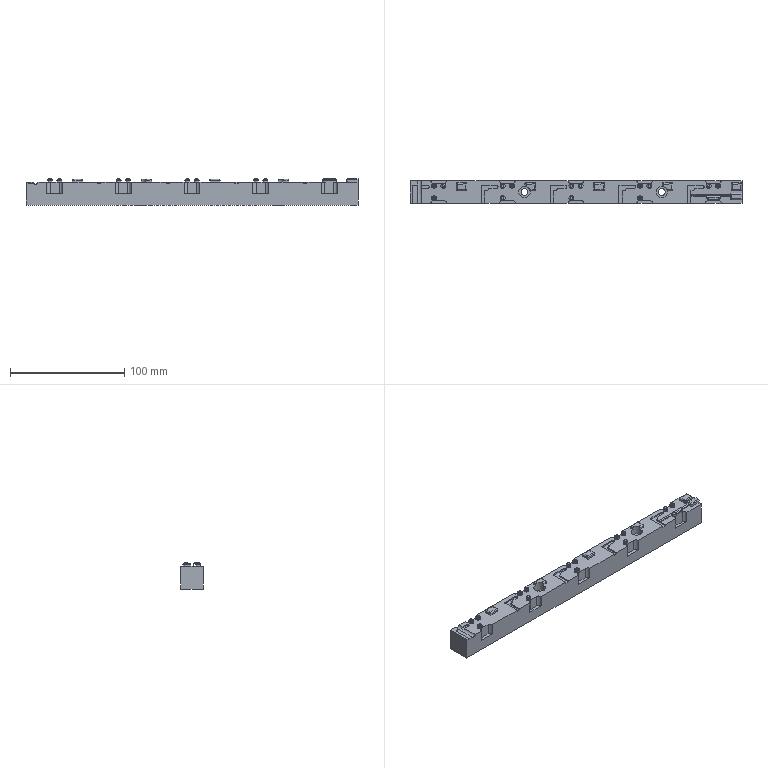Part | STEP file | 01-01 loading base plate | 1 solid | 354 faces | box 290 x 20 x 23 mm | volume 111051 mm3 | plane 131 | cylinder 117 | cone 58 | torus 30 | spline 18 | commonest cylinder face diameters 2 x30 4.2 x28 6 x20 3 x10 5 x8 10 x8